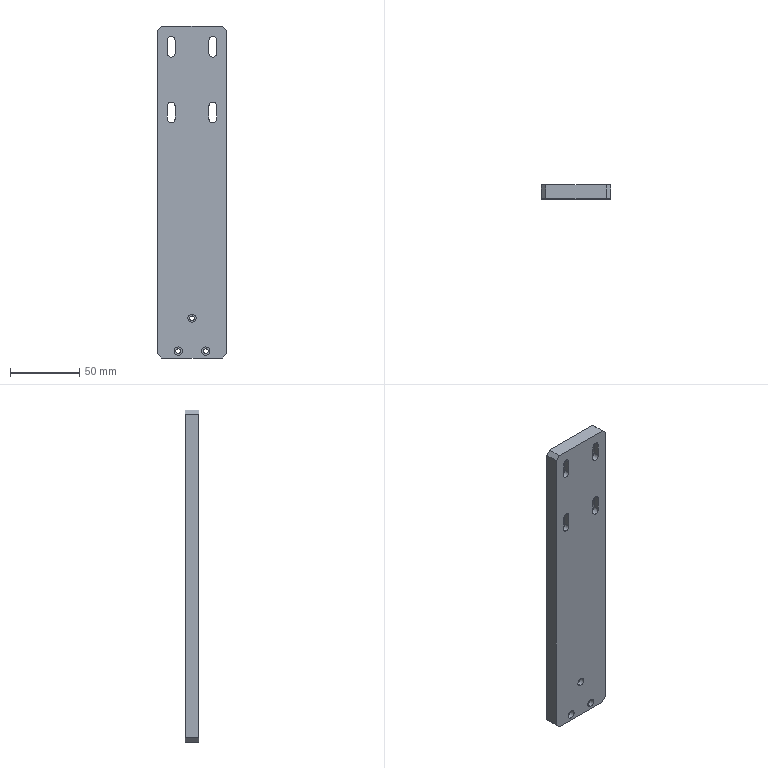Part | SolidWorks | features HoleWzd 2, Chamfer 1, Extrusion 1 | 1 solid | 69 faces | box 50 x 10 x 240 mm | volume 114088 mm3 | cylinder 36 | plane 33 | commonest cylinder face diameters 5.5 x12 10 x12 3.4 x6 6 x6